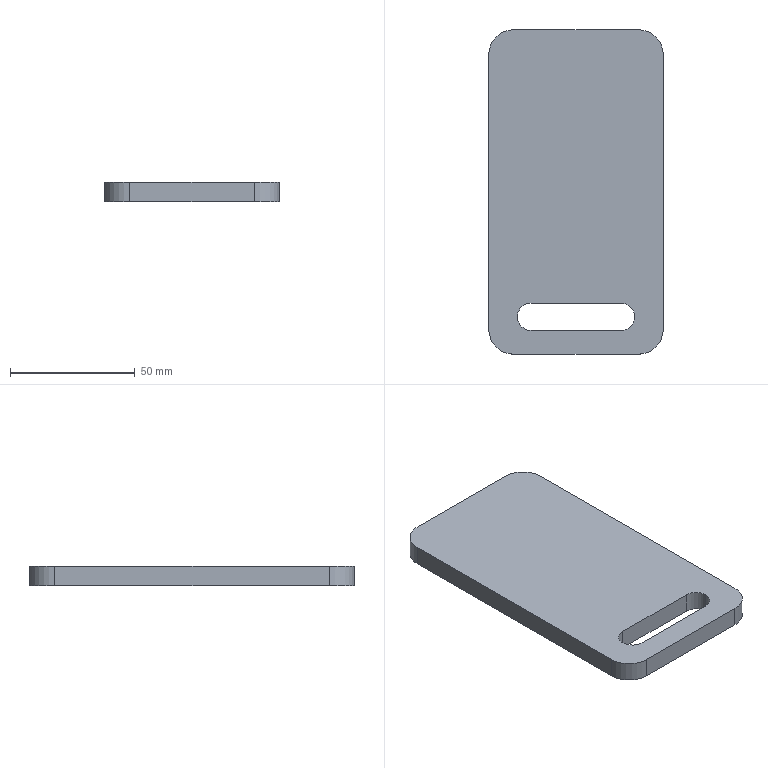Part | SolidWorks | features Extrusion 1, ICE 1 | 1 solid | 15 faces | box 70 x 130 x 8 mm | volume 68185 mm3 | plane 8 | cylinder 7 | commonest cylinder face diameters 20 x4 11 x3
STEP:
#1=CARTESIAN_POINT('',(58.5,15.,0.));
#2=VERTEX_POINT('',#1);
#3=CARTESIAN_POINT('',(53.,20.5,0.));
#4=VERTEX_POINT('',#3);
#5=CARTESIAN_POINT('',(53.,15.,0.));
#6=DIRECTION('',(0.,0.,1.));
#7=DIRECTION('',(1.,0.,0.));
#8=AXIS2_PLACEMENT_3D('',#5,#6,#7);
#9=CIRCLE('',#8,5.5);
#10=EDGE_CURVE('',#2,#4,#9,.T.);
#11=ORIENTED_EDGE('',*,*,#10,.F.);
#12=CARTESIAN_POINT('',(58.5,15.,8.));
#13=VERTEX_POINT('',#12);
#14=CARTESIAN_POINT('',(58.5,15.,-2.));
#15=DIRECTION('',(0.,0.,1.));
#16=VECTOR('',#15,1000.);
#17=LINE('',#14,#16);
#18=EDGE_CURVE('',#2,#13,#17,.T.);
#19=ORIENTED_EDGE('',*,*,#18,.T.);
#20=CARTESIAN_POINT('',(53.,20.5,8.));
#21=VERTEX_POINT('',#20);
#22=CARTESIAN_POINT('',(53.,15.,8.));
#23=DIRECTION('',(0.,0.,1.));
#24=DIRECTION('',(1.,0.,0.));
#25=AXIS2_PLACEMENT_3D('',#22,#23,#24);
#26=CIRCLE('',#25,5.5);
#27=EDGE_CURVE('',#13,#21,#26,.T.);
#28=ORIENTED_EDGE('',*,*,#27,.T.);
#29=CARTESIAN_POINT('',(53.,20.5,-2.));
#30=DIRECTION('',(0.,0.,1.));
#31=VECTOR('',#30,1000.);
#32=LINE('',#29,#31);
#33=EDGE_CURVE('',#4,#21,#32,.T.);
#34=ORIENTED_EDGE('',*,*,#33,.F.);
#35=EDGE_LOOP('',(#11,#19,#28,#34));
#36=FACE_OUTER_BOUND('',#35,.T.);
#37=CARTESIAN_POINT('',(53.,15.,-2.));
#38=DIRECTION('',(0.,0.,1.));
#39=DIRECTION('',(1.,0.,0.));
#40=AXIS2_PLACEMENT_3D('',#37,#38,#39);
#41=CYLINDRICAL_SURFACE('',#40,5.5);
#42=ADVANCED_FACE('',(#36),#41,.F.);
#43=CARTESIAN_POINT('',(70.,120.,0.));
#44=VERTEX_POINT('',#43);
#45=CARTESIAN_POINT('',(60.,130.,0.));
#46=VERTEX_POINT('',#45);
#47=CARTESIAN_POINT('',(60.,120.,0.));
#48=DIRECTION('',(0.,0.,1.));
#49=DIRECTION('',(1.,0.,0.));
#50=AXIS2_PLACEMENT_3D('',#47,#48,#49);
#51=CIRCLE('',#50,10.);
#52=EDGE_CURVE('',#44,#46,#51,.T.);
#53=ORIENTED_EDGE('',*,*,#52,.T.);
#54=CARTESIAN_POINT('',(60.,130.,8.));
#55=VERTEX_POINT('',#54);
#56=CARTESIAN_POINT('',(60.,130.,8.));
#57=DIRECTION('',(0.,0.,-1.));
#58=VECTOR('',#57,1000.);
#59=LINE('',#56,#58);
#60=EDGE_CURVE('',#55,#46,#59,.T.);
#61=ORIENTED_EDGE('',*,*,#60,.F.);
#62=CARTESIAN_POINT('',(70.,120.,8.));
#63=VERTEX_POINT('',#62);
#64=CARTESIAN_POINT('',(60.,120.,8.));
#65=DIRECTION('',(0.,0.,1.));
#66=DIRECTION('',(1.,0.,0.));
#67=AXIS2_PLACEMENT_3D('',#64,#65,#66);
#68=CIRCLE('',#67,10.);
#69=EDGE_CURVE('',#63,#55,#68,.T.);
#70=ORIENTED_EDGE('',*,*,#69,.F.);
#71=CARTESIAN_POINT('',(70.,120.,8.));
#72=DIRECTION('',(0.,0.,-1.));
#73=VECTOR('',#72,1000.);
#74=LINE('',#71,#73);
#75=EDGE_CURVE('',#63,#44,#74,.T.);
#76=ORIENTED_EDGE('',*,*,#75,.T.);
#77=EDGE_LOOP('',(#53,#61,#70,#76));
#78=FACE_OUTER_BOUND('',#77,.T.);
#79=CARTESIAN_POINT('',(60.,120.,8.));
#80=DIRECTION('',(0.,0.,-1.));
#81=DIRECTION('',(-1.,0.,0.));
#82=AXIS2_PLACEMENT_3D('',#79,#80,#81);
#83=CYLINDRICAL_SURFACE('',#82,10.);
#84=ADVANCED_FACE('',(#78),#83,.T.);
#85=CARTESIAN_POINT('',(10.,130.,0.));
#86=VERTEX_POINT('',#85);
#87=CARTESIAN_POINT('',(10.,130.,0.));
#88=DIRECTION('',(-1.,0.,0.));
#89=VECTOR('',#88,1000.);
#90=LINE('',#87,#89);
#91=EDGE_CURVE('',#46,#86,#90,.T.);
#92=ORIENTED_EDGE('',*,*,#91,.T.);
#93=CARTESIAN_POINT('',(10.,130.,8.));
#94=VERTEX_POINT('',#93);
#95=CARTESIAN_POINT('',(10.,130.,8.));
#96=DIRECTION('',(0.,0.,-1.));
#97=VECTOR('',#96,1000.);
#98=LINE('',#95,#97);
#99=EDGE_CURVE('',#94,#86,#98,.T.);
#100=ORIENTED_EDGE('',*,*,#99,.F.);
#101=CARTESIAN_POINT('',(10.,130.,8.));
#102=DIRECTION('',(-1.,0.,0.));
#103=VECTOR('',#102,1000.);
#104=LINE('',#101,#103);
#105=EDGE_CURVE('',#55,#94,#104,.T.);
#106=ORIENTED_EDGE('',*,*,#105,.F.);
#107=ORIENTED_EDGE('',*,*,#60,.T.);
#108=EDGE_LOOP('',(#92,#100,#106,#107));
#109=FACE_OUTER_BOUND('',#108,.T.);
#110=CARTESIAN_POINT('',(10.,130.,8.));
#111=DIRECTION('',(0.,-1.,0.));
#112=DIRECTION('',(0.,0.,-1.));
#113=AXIS2_PLACEMENT_3D('',#110,#111,#112);
#114=PLANE('',#113);
#115=ADVANCED_FACE('',(#109),#114,.F.);
#116=CARTESIAN_POINT('',(0.,120.,0.));
#117=VERTEX_POINT('',#116);
#118=CARTESIAN_POINT('',(10.,120.,0.));
#119=DIRECTION('',(0.,0.,1.));
#120=DIRECTION('',(1.,0.,0.));
#121=AXIS2_PLACEMENT_3D('',#118,#119,#120);
#122=CIRCLE('',#121,10.);
#123=EDGE_CURVE('',#86,#117,#122,.T.);
#124=ORIENTED_EDGE('',*,*,#123,.T.);
#125=CARTESIAN_POINT('',(0.,120.,8.));
#126=VERTEX_POINT('',#125);
#127=CARTESIAN_POINT('',(0.,120.,8.));
#128=DIRECTION('',(0.,0.,-1.));
#129=VECTOR('',#128,1000.);
#130=LINE('',#127,#129);
#131=EDGE_CURVE('',#126,#117,#130,.T.);
#132=ORIENTED_EDGE('',*,*,#131,.F.);
#133=CARTESIAN_POINT('',(10.,120.,8.));
#134=DIRECTION('',(0.,0.,1.));
#135=DIRECTION('',(1.,0.,0.));
#136=AXIS2_PLACEMENT_3D('',#133,#134,#135);
#137=CIRCLE('',#136,10.);
#138=EDGE_CURVE('',#94,#126,#137,.T.);
#139=ORIENTED_EDGE('',*,*,#138,.F.);
#140=ORIENTED_EDGE('',*,*,#99,.T.);
#141=EDGE_LOOP('',(#124,#132,#139,#140));
#142=FACE_OUTER_BOUND('',#141,.T.);
#143=CARTESIAN_POINT('',(10.,120.,8.));
#144=DIRECTION('',(0.,0.,-1.));
#145=DIRECTION('',(-1.,0.,0.));
#146=AXIS2_PLACEMENT_3D('',#143,#144,#145);
#147=CYLINDRICAL_SURFACE('',#146,10.);
#148=ADVANCED_FACE('',(#142),#147,.T.);
#149=CARTESIAN_POINT('',(0.,10.,0.));
#150=VERTEX_POINT('',#149);
#151=CARTESIAN_POINT('',(0.,10.,0.));
#152=DIRECTION('',(0.,-1.,0.));
#153=VECTOR('',#152,1000.);
#154=LINE('',#151,#153);
#155=EDGE_CURVE('',#117,#150,#154,.T.);
#156=ORIENTED_EDGE('',*,*,#155,.T.);
#157=CARTESIAN_POINT('',(0.,10.,8.));
#158=VERTEX_POINT('',#157);
#159=CARTESIAN_POINT('',(0.,10.,8.));
#160=DIRECTION('',(0.,0.,-1.));
#161=VECTOR('',#160,1000.);
#162=LINE('',#159,#161);
#163=EDGE_CURVE('',#158,#150,#162,.T.);
#164=ORIENTED_EDGE('',*,*,#163,.F.);
#165=CARTESIAN_POINT('',(0.,10.,8.));
#166=DIRECTION('',(0.,-1.,0.));
#167=VECTOR('',#166,1000.);
#168=LINE('',#165,#167);
#169=EDGE_CURVE('',#126,#158,#168,.T.);
#170=ORIENTED_EDGE('',*,*,#169,.F.);
#171=ORIENTED_EDGE('',*,*,#131,.T.);
#172=EDGE_LOOP('',(#156,#164,#170,#171));
#173=FACE_OUTER_BOUND('',#172,.T.);
#174=CARTESIAN_POINT('',(0.,10.,8.));
#175=DIRECTION('',(1.,0.,0.));
#176=DIRECTION('',(0.,0.,-1.));
#177=AXIS2_PLACEMENT_3D('',#174,#175,#176);
#178=PLANE('',#177);
#179=ADVANCED_FACE('',(#173),#178,.F.);
#180=CARTESIAN_POINT('',(10.,0.,0.));
#181=VERTEX_POINT('',#180);
#182=CARTESIAN_POINT('',(10.,10.,0.));
#183=DIRECTION('',(0.,0.,1.));
#184=DIRECTION('',(-1.,0.,0.));
#185=AXIS2_PLACEMENT_3D('',#182,#183,#184);
#186=CIRCLE('',#185,10.);
#187=EDGE_CURVE('',#150,#181,#186,.T.);
#188=ORIENTED_EDGE('',*,*,#187,.T.);
#189=CARTESIAN_POINT('',(10.,0.,8.));
#190=VERTEX_POINT('',#189);
#191=CARTESIAN_POINT('',(10.,0.,8.));
#192=DIRECTION('',(0.,0.,-1.));
#193=VECTOR('',#192,1000.);
#194=LINE('',#191,#193);
#195=EDGE_CURVE('',#190,#181,#194,.T.);
#196=ORIENTED_EDGE('',*,*,#195,.F.);
#197=CARTESIAN_POINT('',(10.,10.,8.));
#198=DIRECTION('',(0.,0.,1.));
#199=DIRECTION('',(-1.,0.,0.));
#200=AXIS2_PLACEMENT_3D('',#197,#198,#199);
#201=CIRCLE('',#200,10.);
#202=EDGE_CURVE('',#158,#190,#201,.T.);
#203=ORIENTED_EDGE('',*,*,#202,.F.);
#204=ORIENTED_EDGE('',*,*,#163,.T.);
#205=EDGE_LOOP('',(#188,#196,#203,#204));
#206=FACE_OUTER_BOUND('',#205,.T.);
#207=CARTESIAN_POINT('',(10.,10.,8.));
#208=DIRECTION('',(0.,0.,-1.));
#209=DIRECTION('',(-1.,0.,0.));
#210=AXIS2_PLACEMENT_3D('',#207,#208,#209);
#211=CYLINDRICAL_SURFACE('',#210,10.);
#212=ADVANCED_FACE('',(#206),#211,.T.);
#213=CARTESIAN_POINT('',(60.,0.,0.));
#214=VERTEX_POINT('',#213);
#215=CARTESIAN_POINT('',(10.,0.,0.));
#216=DIRECTION('',(1.,0.,0.));
#217=VECTOR('',#216,1000.);
#218=LINE('',#215,#217);
#219=EDGE_CURVE('',#181,#214,#218,.T.);
#220=ORIENTED_EDGE('',*,*,#219,.T.);
#221=CARTESIAN_POINT('',(60.,0.,8.));
#222=VERTEX_POINT('',#221);
#223=CARTESIAN_POINT('',(60.,0.,8.));
#224=DIRECTION('',(0.,0.,-1.));
#225=VECTOR('',#224,1000.);
#226=LINE('',#223,#225);
#227=EDGE_CURVE('',#222,#214,#226,.T.);
#228=ORIENTED_EDGE('',*,*,#227,.F.);
#229=CARTESIAN_POINT('',(10.,0.,8.));
#230=DIRECTION('',(1.,0.,0.));
#231=VECTOR('',#230,1000.);
#232=LINE('',#229,#231);
#233=EDGE_CURVE('',#190,#222,#232,.T.);
#234=ORIENTED_EDGE('',*,*,#233,.F.);
#235=ORIENTED_EDGE('',*,*,#195,.T.);
#236=EDGE_LOOP('',(#220,#228,#234,#235));
#237=FACE_OUTER_BOUND('',#236,.T.);
#238=CARTESIAN_POINT('',(10.,0.,8.));
#239=DIRECTION('',(0.,1.,0.));
#240=DIRECTION('',(0.,0.,1.));
#241=AXIS2_PLACEMENT_3D('',#238,#239,#240);
#242=PLANE('',#241);
#243=ADVANCED_FACE('',(#237),#242,.F.);
#244=CARTESIAN_POINT('',(70.,10.,0.));
#245=VERTEX_POINT('',#244);
#246=CARTESIAN_POINT('',(60.,10.,0.));
#247=DIRECTION('',(0.,0.,1.));
#248=DIRECTION('',(-1.,0.,0.));
#249=AXIS2_PLACEMENT_3D('',#246,#247,#248);
#250=CIRCLE('',#249,10.);
#251=EDGE_CURVE('',#214,#245,#250,.T.);
#252=ORIENTED_EDGE('',*,*,#251,.T.);
#253=CARTESIAN_POINT('',(70.,10.,8.));
#254=VERTEX_POINT('',#253);
#255=CARTESIAN_POINT('',(70.,10.,8.));
#256=DIRECTION('',(0.,0.,-1.));
#257=VECTOR('',#256,1000.);
#258=LINE('',#255,#257);
#259=EDGE_CURVE('',#254,#245,#258,.T.);
#260=ORIENTED_EDGE('',*,*,#259,.F.);
#261=CARTESIAN_POINT('',(60.,10.,8.));
#262=DIRECTION('',(0.,0.,1.));
#263=DIRECTION('',(-1.,0.,0.));
#264=AXIS2_PLACEMENT_3D('',#261,#262,#263);
#265=CIRCLE('',#264,10.);
#266=EDGE_CURVE('',#222,#254,#265,.T.);
#267=ORIENTED_EDGE('',*,*,#266,.F.);
#268=ORIENTED_EDGE('',*,*,#227,.T.);
#269=EDGE_LOOP('',(#252,#260,#267,#268));
#270=FACE_OUTER_BOUND('',#269,.T.);
#271=CARTESIAN_POINT('',(60.,10.,8.));
#272=DIRECTION('',(0.,0.,-1.));
#273=DIRECTION('',(-1.,0.,0.));
#274=AXIS2_PLACEMENT_3D('',#271,#272,#273);
#275=CYLINDRICAL_SURFACE('',#274,10.);
#276=ADVANCED_FACE('',(#270),#275,.T.);
#277=CARTESIAN_POINT('',(70.,10.,0.));
#278=DIRECTION('',(0.,1.,0.));
#279=VECTOR('',#278,1000.);
#280=LINE('',#277,#279);
#281=EDGE_CURVE('',#245,#44,#280,.T.);
#282=ORIENTED_EDGE('',*,*,#281,.T.);
#283=ORIENTED_EDGE('',*,*,#75,.F.);
#284=CARTESIAN_POINT('',(70.,10.,8.));
#285=DIRECTION('',(0.,1.,0.));
#286=VECTOR('',#285,1000.);
#287=LINE('',#284,#286);
#288=EDGE_CURVE('',#254,#63,#287,.T.);
#289=ORIENTED_EDGE('',*,*,#288,.F.);
#290=ORIENTED_EDGE('',*,*,#259,.T.);
#291=EDGE_LOOP('',(#282,#283,#289,#290));
#292=FACE_OUTER_BOUND('',#291,.T.);
#293=CARTESIAN_POINT('',(70.,10.,8.));
#294=DIRECTION('',(-1.,0.,0.));
#295=DIRECTION('',(0.,0.,1.));
#296=AXIS2_PLACEMENT_3D('',#293,#294,#295);
#297=PLANE('',#296);
#298=ADVANCED_FACE('',(#292),#297,.F.);
#299=CARTESIAN_POINT('',(17.,20.5,8.));
#300=VERTEX_POINT('',#299);
#301=CARTESIAN_POINT('',(17.,9.5,8.));
#302=VERTEX_POINT('',#301);
#303=CARTESIAN_POINT('',(17.,15.,8.));
#304=DIRECTION('',(0.,0.,1.));
#305=DIRECTION('',(1.,0.,0.));
#306=AXIS2_PLACEMENT_3D('',#303,#304,#305);
#307=CIRCLE('',#306,5.5);
#308=EDGE_CURVE('',#300,#302,#307,.T.);
#309=ORIENTED_EDGE('',*,*,#308,.F.);
#310=CARTESIAN_POINT('',(17.,20.5,8.));
#311=DIRECTION('',(-1.,0.,0.));
#312=VECTOR('',#311,1000.);
#313=LINE('',#310,#312);
#314=EDGE_CURVE('',#21,#300,#313,.T.);
#315=ORIENTED_EDGE('',*,*,#314,.F.);
#316=ORIENTED_EDGE('',*,*,#27,.F.);
#317=CARTESIAN_POINT('',(53.,9.5,8.));
#318=VERTEX_POINT('',#317);
#319=CARTESIAN_POINT('',(53.,15.,8.));
#320=DIRECTION('',(0.,0.,1.));
#321=DIRECTION('',(1.,0.,0.));
#322=AXIS2_PLACEMENT_3D('',#319,#320,#321);
#323=CIRCLE('',#322,5.5);
#324=EDGE_CURVE('',#318,#13,#323,.T.);
#325=ORIENTED_EDGE('',*,*,#324,.F.);
#326=CARTESIAN_POINT('',(17.,9.5,8.));
#327=DIRECTION('',(1.,0.,0.));
#328=VECTOR('',#327,1000.);
#329=LINE('',#326,#328);
#330=EDGE_CURVE('',#302,#318,#329,.T.);
#331=ORIENTED_EDGE('',*,*,#330,.F.);
#332=EDGE_LOOP('',(#309,#315,#316,#325,#331));
#333=FACE_BOUND('',#332,.T.);
#334=ORIENTED_EDGE('',*,*,#69,.T.);
#335=ORIENTED_EDGE('',*,*,#105,.T.);
#336=ORIENTED_EDGE('',*,*,#138,.T.);
#337=ORIENTED_EDGE('',*,*,#169,.T.);
#338=ORIENTED_EDGE('',*,*,#202,.T.);
#339=ORIENTED_EDGE('',*,*,#233,.T.);
#340=ORIENTED_EDGE('',*,*,#266,.T.);
#341=ORIENTED_EDGE('',*,*,#288,.T.);
#342=EDGE_LOOP('',(#334,#335,#336,#337,#338,#339,#340,#341));
#343=FACE_OUTER_BOUND('',#342,.T.);
#344=CARTESIAN_POINT('',(60.,120.,8.));
#345=DIRECTION('',(0.,0.,1.));
#346=DIRECTION('',(1.,0.,0.));
#347=AXIS2_PLACEMENT_3D('',#344,#345,#346);
#348=PLANE('',#347);
#349=ADVANCED_FACE('',(#333,#343),#348,.T.);
#350=CARTESIAN_POINT('',(17.,20.5,0.));
#351=VERTEX_POINT('',#350);
#352=CARTESIAN_POINT('',(60.,20.5,0.));
#353=DIRECTION('',(-1.,0.,0.));
#354=VECTOR('',#353,1000.);
#355=LINE('',#352,#354);
#356=EDGE_CURVE('',#4,#351,#355,.T.);
#357=ORIENTED_EDGE('',*,*,#356,.T.);
#358=CARTESIAN_POINT('',(17.,9.5,0.));
#359=VERTEX_POINT('',#358);
#360=CARTESIAN_POINT('',(17.,15.,0.));
#361=DIRECTION('',(0.,0.,1.));
#362=DIRECTION('',(1.,0.,0.));
#363=AXIS2_PLACEMENT_3D('',#360,#361,#362);
#364=CIRCLE('',#363,5.5);
#365=EDGE_CURVE('',#351,#359,#364,.T.);
#366=ORIENTED_EDGE('',*,*,#365,.T.);
#367=CARTESIAN_POINT('',(53.,9.5,0.));
#368=VERTEX_POINT('',#367);
#369=CARTESIAN_POINT('',(60.,9.5,0.));
#370=DIRECTION('',(1.,0.,0.));
#371=VECTOR('',#370,1000.);
#372=LINE('',#369,#371);
#373=EDGE_CURVE('',#359,#368,#372,.T.);
#374=ORIENTED_EDGE('',*,*,#373,.T.);
#375=CARTESIAN_POINT('',(53.,15.,0.));
#376=DIRECTION('',(0.,0.,1.));
#377=DIRECTION('',(1.,0.,0.));
#378=AXIS2_PLACEMENT_3D('',#375,#376,#377);
#379=CIRCLE('',#378,5.5);
#380=EDGE_CURVE('',#368,#2,#379,.T.);
#381=ORIENTED_EDGE('',*,*,#380,.T.);
#382=ORIENTED_EDGE('',*,*,#10,.T.);
#383=EDGE_LOOP('',(#357,#366,#374,#381,#382));
#384=FACE_BOUND('',#383,.T.);
#385=ORIENTED_EDGE('',*,*,#52,.F.);
#386=ORIENTED_EDGE('',*,*,#281,.F.);
#387=ORIENTED_EDGE('',*,*,#251,.F.);
#388=ORIENTED_EDGE('',*,*,#219,.F.);
#389=ORIENTED_EDGE('',*,*,#187,.F.);
#390=ORIENTED_EDGE('',*,*,#155,.F.);
#391=ORIENTED_EDGE('',*,*,#123,.F.);
#392=ORIENTED_EDGE('',*,*,#91,.F.);
#393=EDGE_LOOP('',(#385,#386,#387,#388,#389,#390,#391,#392));
#394=FACE_OUTER_BOUND('',#393,.T.);
#395=CARTESIAN_POINT('',(60.,120.,0.));
#396=DIRECTION('',(0.,0.,1.));
#397=DIRECTION('',(1.,0.,0.));
#398=AXIS2_PLACEMENT_3D('',#395,#396,#397);
#399=PLANE('',#398);
#400=ADVANCED_FACE('',(#384,#394),#399,.F.);
#401=CARTESIAN_POINT('',(17.,20.5,-2.));
#402=DIRECTION('',(0.,0.,1.));
#403=VECTOR('',#402,1000.);
#404=LINE('',#401,#403);
#405=EDGE_CURVE('',#351,#300,#404,.T.);
#406=ORIENTED_EDGE('',*,*,#405,.T.);
#407=ORIENTED_EDGE('',*,*,#308,.T.);
#408=CARTESIAN_POINT('',(17.,9.5,-2.));
#409=DIRECTION('',(0.,0.,1.));
#410=VECTOR('',#409,1000.);
#411=LINE('',#408,#410);
#412=EDGE_CURVE('',#359,#302,#411,.T.);
#413=ORIENTED_EDGE('',*,*,#412,.F.);
#414=ORIENTED_EDGE('',*,*,#365,.F.);
#415=EDGE_LOOP('',(#406,#407,#413,#414));
#416=FACE_OUTER_BOUND('',#415,.T.);
#417=CARTESIAN_POINT('',(17.,15.,-2.));
#418=DIRECTION('',(0.,0.,1.));
#419=DIRECTION('',(1.,0.,0.));
#420=AXIS2_PLACEMENT_3D('',#417,#418,#419);
#421=CYLINDRICAL_SURFACE('',#420,5.5);
#422=ADVANCED_FACE('',(#416),#421,.F.);
#423=ORIENTED_EDGE('',*,*,#33,.T.);
#424=ORIENTED_EDGE('',*,*,#314,.T.);
#425=ORIENTED_EDGE('',*,*,#405,.F.);
#426=ORIENTED_EDGE('',*,*,#356,.F.);
#427=EDGE_LOOP('',(#423,#424,#425,#426));
#428=FACE_OUTER_BOUND('',#427,.T.);
#429=CARTESIAN_POINT('',(17.,20.5,-2.));
#430=DIRECTION('',(0.,1.,0.));
#431=DIRECTION('',(-1.,0.,0.));
#432=AXIS2_PLACEMENT_3D('',#429,#430,#431);
#433=PLANE('',#432);
#434=ADVANCED_FACE('',(#428),#433,.F.);
#435=ORIENTED_EDGE('',*,*,#18,.F.);
#436=ORIENTED_EDGE('',*,*,#380,.F.);
#437=CARTESIAN_POINT('',(53.,9.5,-2.));
#438=DIRECTION('',(0.,0.,1.));
#439=VECTOR('',#438,1000.);
#440=LINE('',#437,#439);
#441=EDGE_CURVE('',#368,#318,#440,.T.);
#442=ORIENTED_EDGE('',*,*,#441,.T.);
#443=ORIENTED_EDGE('',*,*,#324,.T.);
#444=EDGE_LOOP('',(#435,#436,#442,#443));
#445=FACE_OUTER_BOUND('',#444,.T.);
#446=CARTESIAN_POINT('',(53.,15.,-2.));
#447=DIRECTION('',(0.,0.,1.));
#448=DIRECTION('',(1.,0.,0.));
#449=AXIS2_PLACEMENT_3D('',#446,#447,#448);
#450=CYLINDRICAL_SURFACE('',#449,5.5);
#451=ADVANCED_FACE('',(#445),#450,.F.);
#452=ORIENTED_EDGE('',*,*,#412,.T.);
#453=ORIENTED_EDGE('',*,*,#330,.T.);
#454=ORIENTED_EDGE('',*,*,#441,.F.);
#455=ORIENTED_EDGE('',*,*,#373,.F.);
#456=EDGE_LOOP('',(#452,#453,#454,#455));
#457=FACE_OUTER_BOUND('',#456,.T.);
#458=CARTESIAN_POINT('',(17.,9.5,-2.));
#459=DIRECTION('',(0.,-1.,0.));
#460=DIRECTION('',(0.,0.,-1.));
#461=AXIS2_PLACEMENT_3D('',#458,#459,#460);
#462=PLANE('',#461);
#463=ADVANCED_FACE('',(#457),#462,.F.);
#464=CLOSED_SHELL('',(#42,#84,#115,#148,#179,#212,#243,#276,#298,#349,#400,#422,#434,#451,#463));
#465=MANIFOLD_SOLID_BREP('',#464);
#466=CARTESIAN_POINT('',(0.,0.,0.));
#467=DIRECTION('',(0.,0.,1.));
#468=DIRECTION('',(1.,0.,0.));
#469=AXIS2_PLACEMENT_3D('',#466,#467,#468);
#470=(LENGTH_UNIT()NAMED_UNIT(*)SI_UNIT(.MILLI.,.METRE.));
#471=UNCERTAINTY_MEASURE_WITH_UNIT(LENGTH_MEASURE(0.00001),#470,'','');
#472=(NAMED_UNIT(*)PLANE_ANGLE_UNIT()SI_UNIT($,.RADIAN.));
#473=(NAMED_UNIT(*)SI_UNIT($,.STERADIAN.)SOLID_ANGLE_UNIT());
#474=(GEOMETRIC_REPRESENTATION_CONTEXT(3)GLOBAL_UNCERTAINTY_ASSIGNED_CONTEXT((#471))GLOBAL_UNIT_ASSIGNED_CONTEXT((#470,#472,#473))REPRESENTATION_CONTEXT('',''));
#475=ADVANCED_BREP_SHAPE_REPRESENTATION('',(#465,#469),#474);